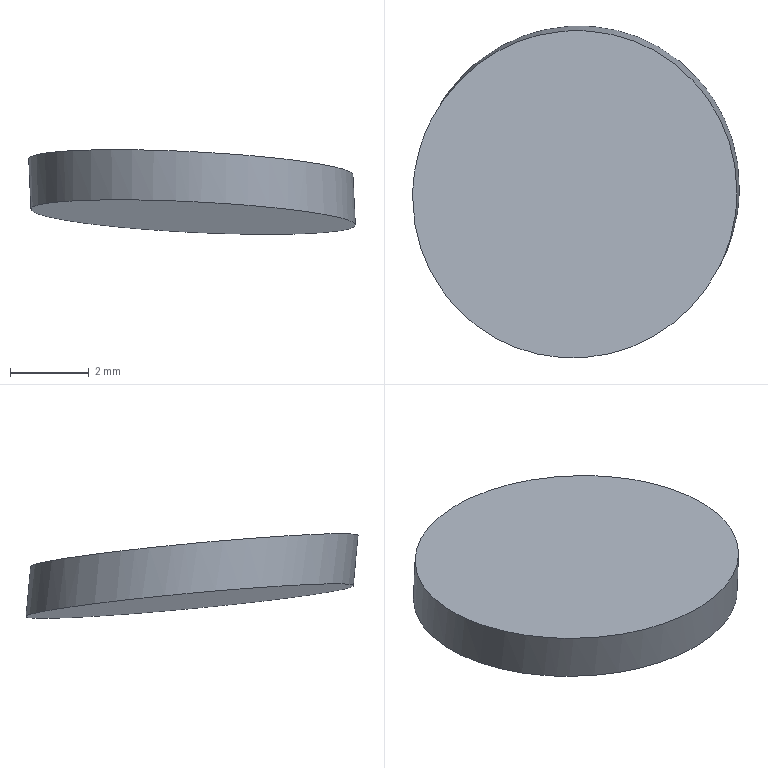Part | STEP file | gslz 2016.10.28-13_id1326_x_t | 1 solid | 3 faces | box 8.284 x 8.42 x 2.147 mm | volume 67.466 mm3 | plane 2 | cylinder 1 | commonest cylinder face diameters 8.2 x1
STEP:
#1=CARTESIAN_POINT('',(0.,0.,0.));
#2=DIRECTION('',(0.,0.,1.));
#3=DIRECTION('',(1.,0.,0.));
#4=AXIS2_PLACEMENT_3D('',#1,#2,#3);
#5=CARTESIAN_POINT('',(1201.289,-23.579,-5.802));
#6=VERTEX_POINT('',#5);
#7=CARTESIAN_POINT('',(1193.983,-19.857,-5.802));
#8=VERTEX_POINT('',#7);
#9=CARTESIAN_POINT('',(1201.289,-23.579,-5.802));
#10=CARTESIAN_POINT('',(1200.799,-24.541,-5.688));
#11=CARTESIAN_POINT('',(1199.927,-25.305,-5.575));
#12=CARTESIAN_POINT('',(1197.878,-26.002,-5.412));
#13=CARTESIAN_POINT('',(1196.71,-25.925,-5.364));
#14=CARTESIAN_POINT('',(1194.776,-24.94,-5.364));
#15=CARTESIAN_POINT('',(1194.028,-24.041,-5.412));
#16=CARTESIAN_POINT('',(1193.387,-21.973,-5.575));
#17=CARTESIAN_POINT('',(1193.493,-20.819,-5.688));
#18=CARTESIAN_POINT('',(1193.983,-19.857,-5.802));
#19=B_SPLINE_CURVE_WITH_KNOTS('',3,(#9,#10,#11,#12,#13,#14,#15,#16,#17,#18),.UNSPECIFIED.,.F.,.F.,(4,2,2,2,4),(0.,0.25,0.5,0.75,1.),.UNSPECIFIED.);
#20=CARTESIAN_POINT('',(1199.529,-18.002,-6.24));
#21=DIRECTION('',(-0.04745,-0.09314,-0.9945));
#22=DIRECTION('',(0.,0.9956,-0.09324));
#23=AXIS2_PLACEMENT_3D('',#20,#21,#22);
#24=PLANE('',#23);
#25=CARTESIAN_POINT('',(-5.594,1.762));
#26=CARTESIAN_POINT('',(-6.562,1.271));
#27=CARTESIAN_POINT('',(-7.333,0.3981));
#28=CARTESIAN_POINT('',(-8.043,-1.653));
#29=CARTESIAN_POINT('',(-7.97,-2.822));
#30=CARTESIAN_POINT('',(-6.989,-4.758));
#31=CARTESIAN_POINT('',(-6.09,-5.508));
#32=CARTESIAN_POINT('',(-4.016,-6.149));
#33=CARTESIAN_POINT('',(-2.856,-6.044));
#34=CARTESIAN_POINT('',(-1.888,-5.553));
#35=B_SPLINE_CURVE_WITH_KNOTS('',3,(#25,#26,#27,#28,#29,#30,#31,#32,#33,#34),.UNSPECIFIED.,.F.,.F.,(4,2,2,2,4),(0.,0.25,0.5,0.75,1.),.UNSPECIFIED.);
#36=(GEOMETRIC_REPRESENTATION_CONTEXT(2)PARAMETRIC_REPRESENTATION_CONTEXT()REPRESENTATION_CONTEXT('',''));
#37=DEFINITIONAL_REPRESENTATION('',(#35),#36);
#38=PCURVE('',#24,#37);
#39=CARTESIAN_POINT('',(1197.636,-21.718,-5.802));
#40=DIRECTION('',(0.04745,0.09314,-0.9945));
#41=DIRECTION('',(-0.891,0.454,0.));
#42=AXIS2_PLACEMENT_3D('',#39,#40,#41);
#43=CYLINDRICAL_SURFACE('',#42,4.1);
#44=CARTESIAN_POINT('',(3.142,0.));
#45=CARTESIAN_POINT('',(3.189,-0.04103));
#46=CARTESIAN_POINT('',(3.283,-0.123));
#47=CARTESIAN_POINT('',(3.424,-0.2437));
#48=CARTESIAN_POINT('',(3.566,-0.3597));
#49=CARTESIAN_POINT('',(3.708,-0.4689));
#50=CARTESIAN_POINT('',(3.85,-0.569));
#51=CARTESIAN_POINT('',(3.993,-0.6577));
#52=CARTESIAN_POINT('',(4.136,-0.7327));
#53=CARTESIAN_POINT('',(4.28,-0.793));
#54=CARTESIAN_POINT('',(4.424,-0.8375));
#55=CARTESIAN_POINT('',(4.568,-0.8651));
#56=CARTESIAN_POINT('',(4.712,-0.8747));
#57=CARTESIAN_POINT('',(4.857,-0.8651));
#58=CARTESIAN_POINT('',(5.001,-0.8375));
#59=CARTESIAN_POINT('',(5.145,-0.793));
#60=CARTESIAN_POINT('',(5.289,-0.7327));
#61=CARTESIAN_POINT('',(5.432,-0.6577));
#62=CARTESIAN_POINT('',(5.575,-0.569));
#63=CARTESIAN_POINT('',(5.717,-0.4689));
#64=CARTESIAN_POINT('',(5.859,-0.3597));
#65=CARTESIAN_POINT('',(6.001,-0.2437));
#66=CARTESIAN_POINT('',(6.142,-0.123));
#67=CARTESIAN_POINT('',(6.236,-0.04103));
#68=CARTESIAN_POINT('',(6.283,0.));
#69=B_SPLINE_CURVE_WITH_KNOTS('',3,(#44,#45,#46,#47,#48,#49,#50,#51,#52,#53,#54,#55,#56,#57,#58,#59,#60,#61,#62,#63,#64,#65,#66,#67,#68),.UNSPECIFIED.,.F.,.F.,(4,1,1,1,1,1,1,1,1,1,1,1,1,1,1,1,1,1,1,1,1,1,4),(0.,0.04545,0.09091,0.1364,0.1818,0.2273,0.2727,0.3182,0.3636,0.4091,0.4545,0.5,0.5455,0.5909,0.6364,0.6818,0.7273,0.7727,0.8182,0.8636,0.9091,0.9545,1.),.QUASI_UNIFORM_KNOTS.);
#70=(GEOMETRIC_REPRESENTATION_CONTEXT(2)PARAMETRIC_REPRESENTATION_CONTEXT()REPRESENTATION_CONTEXT('',''));
#71=DEFINITIONAL_REPRESENTATION('',(#69),#70);
#72=PCURVE('',#43,#71);
#73=SURFACE_CURVE('',#19,(#38,#72),.PCURVE_S1.);
#74=EDGE_CURVE('',#6,#8,#73,.T.);
#75=ORIENTED_EDGE('',*,*,#74,.F.);
#76=CARTESIAN_POINT('',(1193.983,-19.857,-5.802));
#77=CARTESIAN_POINT('',(1194.473,-18.895,-5.915));
#78=CARTESIAN_POINT('',(1195.345,-18.131,-6.028));
#79=CARTESIAN_POINT('',(1197.394,-17.434,-6.192));
#80=CARTESIAN_POINT('',(1198.561,-17.511,-6.24));
#81=CARTESIAN_POINT('',(1200.495,-18.497,-6.24));
#82=CARTESIAN_POINT('',(1201.244,-19.396,-6.192));
#83=CARTESIAN_POINT('',(1201.884,-21.463,-6.029));
#84=CARTESIAN_POINT('',(1201.779,-22.618,-5.915));
#85=CARTESIAN_POINT('',(1201.289,-23.579,-5.802));
#86=B_SPLINE_CURVE_WITH_KNOTS('',3,(#76,#77,#78,#79,#80,#81,#82,#83,#84,#85),.UNSPECIFIED.,.F.,.F.,(4,2,2,2,4),(0.,0.25,0.5,0.75,1.),.UNSPECIFIED.);
#87=CARTESIAN_POINT('',(-1.888,-5.553));
#88=CARTESIAN_POINT('',(-0.9195,-5.062));
#89=CARTESIAN_POINT('',(-0.1488,-4.189));
#90=CARTESIAN_POINT('',(0.5607,-2.138));
#91=CARTESIAN_POINT('',(0.4886,-0.9692));
#92=CARTESIAN_POINT('',(-0.4925,0.9671));
#93=CARTESIAN_POINT('',(-1.392,1.716));
#94=CARTESIAN_POINT('',(-3.466,2.358));
#95=CARTESIAN_POINT('',(-4.626,2.252));
#96=CARTESIAN_POINT('',(-5.594,1.762));
#97=B_SPLINE_CURVE_WITH_KNOTS('',3,(#87,#88,#89,#90,#91,#92,#93,#94,#95,#96),.UNSPECIFIED.,.F.,.F.,(4,2,2,2,4),(0.,0.25,0.5,0.75,1.),.UNSPECIFIED.);
#98=(GEOMETRIC_REPRESENTATION_CONTEXT(2)PARAMETRIC_REPRESENTATION_CONTEXT()REPRESENTATION_CONTEXT('',''));
#99=DEFINITIONAL_REPRESENTATION('',(#97),#98);
#100=PCURVE('',#24,#99);
#101=CARTESIAN_POINT('',(0.,0.));
#102=CARTESIAN_POINT('',(0.04706,0.04103));
#103=CARTESIAN_POINT('',(0.1412,0.123));
#104=CARTESIAN_POINT('',(0.2826,0.2437));
#105=CARTESIAN_POINT('',(0.4244,0.3597));
#106=CARTESIAN_POINT('',(0.5663,0.4689));
#107=CARTESIAN_POINT('',(0.7085,0.569));
#108=CARTESIAN_POINT('',(0.8512,0.6577));
#109=CARTESIAN_POINT('',(0.9945,0.7327));
#110=CARTESIAN_POINT('',(1.138,0.793));
#111=CARTESIAN_POINT('',(1.282,0.8375));
#112=CARTESIAN_POINT('',(1.427,0.8651));
#113=CARTESIAN_POINT('',(1.571,0.8747));
#114=CARTESIAN_POINT('',(1.715,0.8651));
#115=CARTESIAN_POINT('',(1.859,0.8375));
#116=CARTESIAN_POINT('',(2.003,0.793));
#117=CARTESIAN_POINT('',(2.147,0.7327));
#118=CARTESIAN_POINT('',(2.29,0.6577));
#119=CARTESIAN_POINT('',(2.433,0.569));
#120=CARTESIAN_POINT('',(2.575,0.4689));
#121=CARTESIAN_POINT('',(2.717,0.3597));
#122=CARTESIAN_POINT('',(2.859,0.2437));
#123=CARTESIAN_POINT('',(3.,0.123));
#124=CARTESIAN_POINT('',(3.095,0.04103));
#125=CARTESIAN_POINT('',(3.142,0.));
#126=B_SPLINE_CURVE_WITH_KNOTS('',3,(#101,#102,#103,#104,#105,#106,#107,#108,#109,#110,#111,#112,#113,#114,#115,#116,#117,#118,#119,#120,#121,#122,#123,#124,#125),.UNSPECIFIED.,.F.,.F.,(4,1,1,1,1,1,1,1,1,1,1,1,1,1,1,1,1,1,1,1,1,1,4),(0.,0.04545,0.09091,0.1364,0.1818,0.2273,0.2727,0.3182,0.3636,0.4091,0.4545,0.5,0.5455,0.5909,0.6364,0.6818,0.7273,0.7727,0.8182,0.8636,0.9091,0.9545,1.),.QUASI_UNIFORM_KNOTS.);
#127=(GEOMETRIC_REPRESENTATION_CONTEXT(2)PARAMETRIC_REPRESENTATION_CONTEXT()REPRESENTATION_CONTEXT('',''));
#128=DEFINITIONAL_REPRESENTATION('',(#126),#127);
#129=PCURVE('',#43,#128);
#130=SURFACE_CURVE('',#86,(#100,#129),.PCURVE_S1.);
#131=EDGE_CURVE('',#8,#6,#130,.T.);
#132=ORIENTED_EDGE('',*,*,#131,.F.);
#133=EDGE_LOOP('',(#75,#132));
#134=FACE_BOUND('',#133,.T.);
#135=ADVANCED_FACE('',(#134),#24,.F.);
#136=ORIENTED_EDGE('',*,*,#131,.T.);
#137=ORIENTED_EDGE('',*,*,#74,.T.);
#138=CARTESIAN_POINT('',(1194.043,-19.738,-7.073));
#139=VERTEX_POINT('',#138);
#140=CARTESIAN_POINT('',(1193.983,-19.857,-5.802));
#141=CARTESIAN_POINT('',(1194.043,-19.738,-7.073));
#142=B_SPLINE_CURVE_WITH_KNOTS('',1,(#140,#141),.UNSPECIFIED.,.F.,.F.,(2,2),(0.,1.278),.PIECEWISE_BEZIER_KNOTS.);
#143=CARTESIAN_POINT('',(6.283,0.));
#144=DIRECTION('',(0.,1.));
#145=VECTOR('',#144,1.);
#146=LINE('',#143,#145);
#147=(GEOMETRIC_REPRESENTATION_CONTEXT(2)PARAMETRIC_REPRESENTATION_CONTEXT()REPRESENTATION_CONTEXT('',''));
#148=DEFINITIONAL_REPRESENTATION('',(#146),#147);
#149=PCURVE('',#43,#148);
#150=CARTESIAN_POINT('',(0.,0.));
#151=DIRECTION('',(0.,1.));
#152=VECTOR('',#151,1.);
#153=LINE('',#150,#152);
#154=(GEOMETRIC_REPRESENTATION_CONTEXT(2)PARAMETRIC_REPRESENTATION_CONTEXT()REPRESENTATION_CONTEXT('',''));
#155=DEFINITIONAL_REPRESENTATION('',(#153),#154);
#156=PCURVE('',#43,#155);
#157=SEAM_CURVE('',#142,(#149,#156),.PCURVE_S1.);
#158=EDGE_CURVE('',#8,#139,#157,.T.);
#159=ORIENTED_EDGE('',*,*,#158,.T.);
#160=CARTESIAN_POINT('',(1201.349,-23.46,-7.073));
#161=VERTEX_POINT('',#160);
#162=CARTESIAN_POINT('',(1201.349,-23.46,-7.073));
#163=CARTESIAN_POINT('',(1200.857,-24.427,-6.959));
#164=CARTESIAN_POINT('',(1199.987,-25.186,-6.846));
#165=CARTESIAN_POINT('',(1197.938,-25.883,-6.683));
#166=CARTESIAN_POINT('',(1196.772,-25.807,-6.635));
#167=CARTESIAN_POINT('',(1194.835,-24.82,-6.635));
#168=CARTESIAN_POINT('',(1194.09,-23.926,-6.683));
#169=CARTESIAN_POINT('',(1193.447,-21.85,-6.847));
#170=CARTESIAN_POINT('',(1193.551,-20.704,-6.959));
#171=CARTESIAN_POINT('',(1194.043,-19.738,-7.073));
#172=B_SPLINE_CURVE_WITH_KNOTS('',3,(#162,#163,#164,#165,#166,#167,#168,#169,#170,#171),.UNSPECIFIED.,.F.,.F.,(4,2,2,2,4),(0.,0.25,0.5,0.75,1.),.UNSPECIFIED.);
#173=CARTESIAN_POINT('',(3.142,1.278));
#174=CARTESIAN_POINT('',(3.189,1.237));
#175=CARTESIAN_POINT('',(3.283,1.154));
#176=CARTESIAN_POINT('',(3.425,1.034));
#177=CARTESIAN_POINT('',(3.566,0.9178));
#178=CARTESIAN_POINT('',(3.708,0.8088));
#179=CARTESIAN_POINT('',(3.85,0.7089));
#180=CARTESIAN_POINT('',(3.993,0.6203));
#181=CARTESIAN_POINT('',(4.136,0.5453));
#182=CARTESIAN_POINT('',(4.28,0.4849));
#183=CARTESIAN_POINT('',(4.424,0.4404));
#184=CARTESIAN_POINT('',(4.568,0.4128));
#185=CARTESIAN_POINT('',(4.712,0.4033));
#186=CARTESIAN_POINT('',(4.857,0.4128));
#187=CARTESIAN_POINT('',(5.001,0.4403));
#188=CARTESIAN_POINT('',(5.145,0.4846));
#189=CARTESIAN_POINT('',(5.288,0.5449));
#190=CARTESIAN_POINT('',(5.432,0.62));
#191=CARTESIAN_POINT('',(5.575,0.7091));
#192=CARTESIAN_POINT('',(5.717,0.8092));
#193=CARTESIAN_POINT('',(5.859,0.9182));
#194=CARTESIAN_POINT('',(6.,1.034));
#195=CARTESIAN_POINT('',(6.142,1.155));
#196=CARTESIAN_POINT('',(6.236,1.237));
#197=CARTESIAN_POINT('',(6.283,1.278));
#198=B_SPLINE_CURVE_WITH_KNOTS('',3,(#173,#174,#175,#176,#177,#178,#179,#180,#181,#182,#183,#184,#185,#186,#187,#188,#189,#190,#191,#192,#193,#194,#195,#196,#197),.UNSPECIFIED.,.F.,.F.,(4,1,1,1,1,1,1,1,1,1,1,1,1,1,1,1,1,1,1,1,1,1,4),(0.,0.04545,0.09091,0.1364,0.1818,0.2273,0.2727,0.3182,0.3636,0.4091,0.4545,0.5,0.5455,0.5909,0.6364,0.6818,0.7273,0.7727,0.8182,0.8636,0.9091,0.9545,1.),.QUASI_UNIFORM_KNOTS.);
#199=(GEOMETRIC_REPRESENTATION_CONTEXT(2)PARAMETRIC_REPRESENTATION_CONTEXT()REPRESENTATION_CONTEXT('',''));
#200=DEFINITIONAL_REPRESENTATION('',(#198),#199);
#201=PCURVE('',#43,#200);
#202=CARTESIAN_POINT('',(1199.47,-18.118,-7.483));
#203=DIRECTION('',(-0.04745,-0.09314,-0.9945));
#204=DIRECTION('',(0.,0.9956,-0.09324));
#205=AXIS2_PLACEMENT_3D('',#202,#203,#204);
#206=PLANE('',#205);
#207=CARTESIAN_POINT('',(-5.357,1.882));
#208=CARTESIAN_POINT('',(-6.33,1.388));
#209=CARTESIAN_POINT('',(-7.096,0.518));
#210=CARTESIAN_POINT('',(-7.805,-1.533));
#211=CARTESIAN_POINT('',(-7.734,-2.7));
#212=CARTESIAN_POINT('',(-6.751,-4.64));
#213=CARTESIAN_POINT('',(-5.857,-5.386));
#214=CARTESIAN_POINT('',(-3.774,-6.03));
#215=CARTESIAN_POINT('',(-2.623,-5.925));
#216=CARTESIAN_POINT('',(-1.651,-5.433));
#217=B_SPLINE_CURVE_WITH_KNOTS('',3,(#207,#208,#209,#210,#211,#212,#213,#214,#215,#216),.UNSPECIFIED.,.F.,.F.,(4,2,2,2,4),(0.,0.25,0.5,0.75,1.),.UNSPECIFIED.);
#218=(GEOMETRIC_REPRESENTATION_CONTEXT(2)PARAMETRIC_REPRESENTATION_CONTEXT()REPRESENTATION_CONTEXT('',''));
#219=DEFINITIONAL_REPRESENTATION('',(#217),#218);
#220=PCURVE('',#206,#219);
#221=SURFACE_CURVE('',#172,(#201,#220),.PCURVE_S1.);
#222=EDGE_CURVE('',#161,#139,#221,.T.);
#223=ORIENTED_EDGE('',*,*,#222,.F.);
#224=CARTESIAN_POINT('',(1194.043,-19.738,-7.073));
#225=CARTESIAN_POINT('',(1194.536,-18.771,-7.187));
#226=CARTESIAN_POINT('',(1195.405,-18.012,-7.299));
#227=CARTESIAN_POINT('',(1197.454,-17.315,-7.462));
#228=CARTESIAN_POINT('',(1198.62,-17.391,-7.511));
#229=CARTESIAN_POINT('',(1200.557,-18.378,-7.511));
#230=CARTESIAN_POINT('',(1201.303,-19.272,-7.463));
#231=CARTESIAN_POINT('',(1201.946,-21.349,-7.299));
#232=CARTESIAN_POINT('',(1201.841,-22.495,-7.187));
#233=CARTESIAN_POINT('',(1201.349,-23.46,-7.073));
#234=B_SPLINE_CURVE_WITH_KNOTS('',3,(#224,#225,#226,#227,#228,#229,#230,#231,#232,#233),.UNSPECIFIED.,.F.,.F.,(4,2,2,2,4),(0.,0.25,0.5,0.75,1.),.UNSPECIFIED.);
#235=CARTESIAN_POINT('',(0.,1.278));
#236=CARTESIAN_POINT('',(0.04732,1.319));
#237=CARTESIAN_POINT('',(0.1418,1.401));
#238=CARTESIAN_POINT('',(0.2833,1.522));
#239=CARTESIAN_POINT('',(0.4249,1.638));
#240=CARTESIAN_POINT('',(0.5666,1.747));
#241=CARTESIAN_POINT('',(0.7085,1.847));
#242=CARTESIAN_POINT('',(0.8512,1.936));
#243=CARTESIAN_POINT('',(0.9944,2.011));
#244=CARTESIAN_POINT('',(1.138,2.071));
#245=CARTESIAN_POINT('',(1.282,2.115));
#246=CARTESIAN_POINT('',(1.426,2.143));
#247=CARTESIAN_POINT('',(1.571,2.153));
#248=CARTESIAN_POINT('',(1.715,2.143));
#249=CARTESIAN_POINT('',(1.859,2.116));
#250=CARTESIAN_POINT('',(2.003,2.071));
#251=CARTESIAN_POINT('',(2.147,2.011));
#252=CARTESIAN_POINT('',(2.29,1.936));
#253=CARTESIAN_POINT('',(2.433,1.847));
#254=CARTESIAN_POINT('',(2.576,1.747));
#255=CARTESIAN_POINT('',(2.717,1.638));
#256=CARTESIAN_POINT('',(2.859,1.522));
#257=CARTESIAN_POINT('',(3.,1.401));
#258=CARTESIAN_POINT('',(3.094,1.319));
#259=CARTESIAN_POINT('',(3.142,1.278));
#260=B_SPLINE_CURVE_WITH_KNOTS('',3,(#235,#236,#237,#238,#239,#240,#241,#242,#243,#244,#245,#246,#247,#248,#249,#250,#251,#252,#253,#254,#255,#256,#257,#258,#259),.UNSPECIFIED.,.F.,.F.,(4,1,1,1,1,1,1,1,1,1,1,1,1,1,1,1,1,1,1,1,1,1,4),(0.,0.04545,0.09091,0.1364,0.1818,0.2273,0.2727,0.3182,0.3636,0.4091,0.4545,0.5,0.5455,0.5909,0.6364,0.6818,0.7273,0.7727,0.8182,0.8636,0.9091,0.9545,1.),.QUASI_UNIFORM_KNOTS.);
#261=(GEOMETRIC_REPRESENTATION_CONTEXT(2)PARAMETRIC_REPRESENTATION_CONTEXT()REPRESENTATION_CONTEXT('',''));
#262=DEFINITIONAL_REPRESENTATION('',(#260),#261);
#263=PCURVE('',#43,#262);
#264=CARTESIAN_POINT('',(-1.651,-5.433));
#265=CARTESIAN_POINT('',(-0.6773,-4.939));
#266=CARTESIAN_POINT('',(0.08844,-4.069));
#267=CARTESIAN_POINT('',(0.7975,-2.018));
#268=CARTESIAN_POINT('',(0.7266,-0.8506));
#269=CARTESIAN_POINT('',(-0.2565,1.089));
#270=CARTESIAN_POINT('',(-1.151,1.835));
#271=CARTESIAN_POINT('',(-3.233,2.479));
#272=CARTESIAN_POINT('',(-4.385,2.374));
#273=CARTESIAN_POINT('',(-5.357,1.882));
#274=B_SPLINE_CURVE_WITH_KNOTS('',3,(#264,#265,#266,#267,#268,#269,#270,#271,#272,#273),.UNSPECIFIED.,.F.,.F.,(4,2,2,2,4),(0.,0.25,0.5,0.75,1.),.UNSPECIFIED.);
#275=(GEOMETRIC_REPRESENTATION_CONTEXT(2)PARAMETRIC_REPRESENTATION_CONTEXT()REPRESENTATION_CONTEXT('',''));
#276=DEFINITIONAL_REPRESENTATION('',(#274),#275);
#277=PCURVE('',#206,#276);
#278=SURFACE_CURVE('',#234,(#263,#277),.PCURVE_S1.);
#279=EDGE_CURVE('',#139,#161,#278,.T.);
#280=ORIENTED_EDGE('',*,*,#279,.F.);
#281=ORIENTED_EDGE('',*,*,#158,.F.);
#282=EDGE_LOOP('',(#136,#137,#159,#223,#280,#281));
#283=FACE_BOUND('',#282,.T.);
#284=ADVANCED_FACE('',(#283),#43,.T.);
#285=ORIENTED_EDGE('',*,*,#279,.T.);
#286=ORIENTED_EDGE('',*,*,#222,.T.);
#287=EDGE_LOOP('',(#285,#286));
#288=FACE_BOUND('',#287,.T.);
#289=ADVANCED_FACE('',(#288),#206,.T.);
#290=CLOSED_SHELL('',(#135,#284,#289));
#291=MANIFOLD_SOLID_BREP('',#290);
#292=(LENGTH_UNIT()NAMED_UNIT(*)SI_UNIT(.MILLI.,.METRE.));
#293=UNCERTAINTY_MEASURE_WITH_UNIT(LENGTH_MEASURE(0.005),#292,'','');
#294=(NAMED_UNIT(*)PLANE_ANGLE_UNIT()SI_UNIT($,.RADIAN.));
#295=(NAMED_UNIT(*)SI_UNIT($,.STERADIAN.)SOLID_ANGLE_UNIT());
#296=(GEOMETRIC_REPRESENTATION_CONTEXT(3)GLOBAL_UNCERTAINTY_ASSIGNED_CONTEXT((#293))GLOBAL_UNIT_ASSIGNED_CONTEXT((#292,#294,#295))REPRESENTATION_CONTEXT('',''));
#297=ADVANCED_BREP_SHAPE_REPRESENTATION('',(#4,#291),#296);